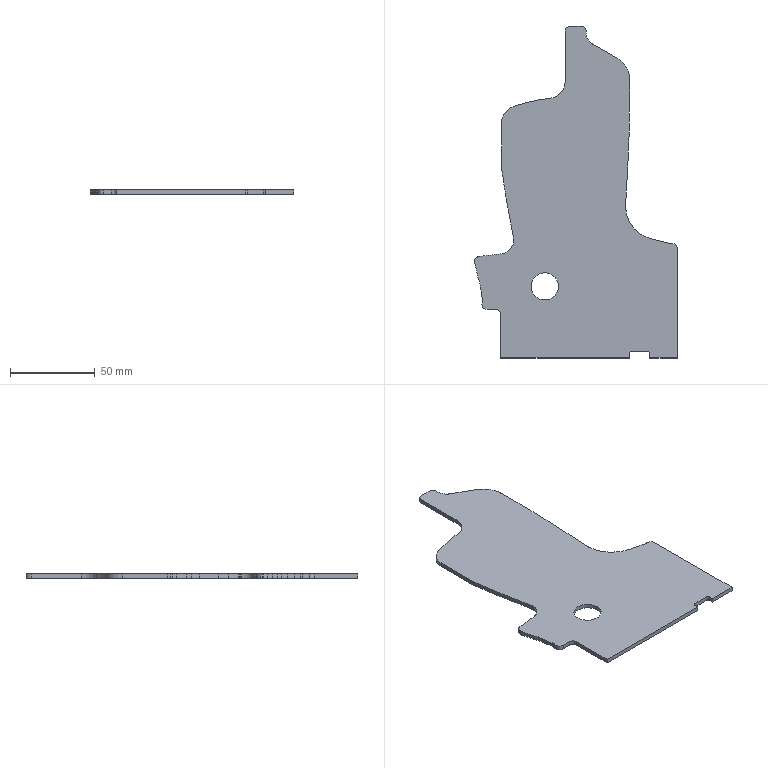Part | STEP file | lll_id1250_x_t | 1 solid | 83 faces | box 119.869 x 195.891 x 2.5 mm | volume 36599 mm3 | cylinder 68 | plane 15 | commonest cylinder face diameters 6 x7 2 x2 20 x2 5.009 x1 5.158 x1 5.699 x1